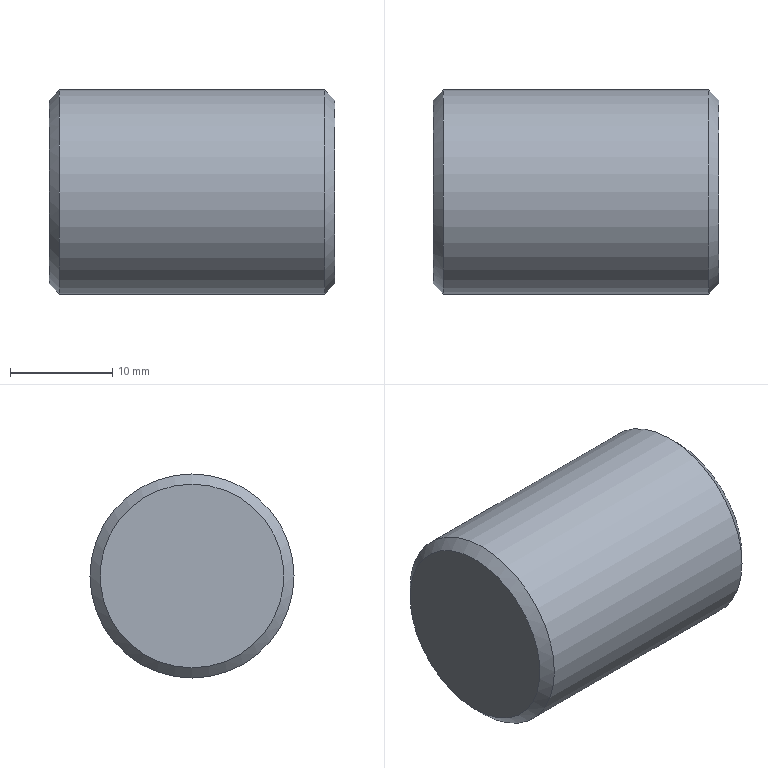Part | NX | features DATUM_CSYS 2, CHAMFER 1, EXTRUDE 1, SKETCH 1 | 1 solid | 5 faces | box 28 x 20 x 20 mm | volume 8736 mm3 | plane 2 | cone 2 | cylinder 1 | commonest cylinder face diameters 20 x1
STEP:
#1=CARTESIAN_POINT('',(-13.,0.,-10.));
#2=VERTEX_POINT('',#1);
#3=CARTESIAN_POINT('',(-13.,0.,0.));
#4=DIRECTION('',(1.,0.,0.));
#5=DIRECTION('',(0.,0.,-1.));
#6=AXIS2_PLACEMENT_3D('',#3,#4,#5);
#7=CIRCLE('',#6,10.);
#8=EDGE_CURVE('',#2,#2,#7,.T.);
#9=ORIENTED_EDGE('',*,*,#8,.T.);
#10=EDGE_LOOP('',(#9));
#11=FACE_BOUND('',#10,.T.);
#12=CARTESIAN_POINT('',(13.,0.,-10.));
#13=VERTEX_POINT('',#12);
#14=CARTESIAN_POINT('',(13.,0.,0.));
#15=DIRECTION('',(1.,0.,0.));
#16=DIRECTION('',(0.,0.,-1.));
#17=AXIS2_PLACEMENT_3D('',#14,#15,#16);
#18=CIRCLE('',#17,10.);
#19=EDGE_CURVE('',#13,#13,#18,.F.);
#20=ORIENTED_EDGE('',*,*,#19,.T.);
#21=EDGE_LOOP('',(#20));
#22=FACE_BOUND('',#21,.T.);
#23=CARTESIAN_POINT('',(14.,0.,0.));
#24=DIRECTION('',(-1.,0.,0.));
#25=DIRECTION('',(0.,0.,1.));
#26=AXIS2_PLACEMENT_3D('',#23,#24,#25);
#27=CYLINDRICAL_SURFACE('',#26,10.);
#28=ADVANCED_FACE('',(#11,#22),#27,.T.);
#29=CARTESIAN_POINT('',(14.,0.,-9.));
#30=VERTEX_POINT('',#29);
#31=CARTESIAN_POINT('',(14.,0.,0.));
#32=DIRECTION('',(1.,0.,0.));
#33=DIRECTION('',(0.,0.,-1.));
#34=AXIS2_PLACEMENT_3D('',#31,#32,#33);
#35=CIRCLE('',#34,9.);
#36=EDGE_CURVE('',#30,#30,#35,.T.);
#37=ORIENTED_EDGE('',*,*,#36,.T.);
#38=EDGE_LOOP('',(#37));
#39=FACE_BOUND('',#38,.T.);
#40=CARTESIAN_POINT('',(14.,0.,0.));
#41=DIRECTION('',(1.,0.,0.));
#42=DIRECTION('',(0.,0.,-1.));
#43=AXIS2_PLACEMENT_3D('',#40,#41,#42);
#44=PLANE('',#43);
#45=ADVANCED_FACE('',(#39),#44,.T.);
#46=CARTESIAN_POINT('',(-14.,0.,-9.));
#47=VERTEX_POINT('',#46);
#48=CARTESIAN_POINT('',(-14.,0.,0.));
#49=DIRECTION('',(1.,0.,0.));
#50=DIRECTION('',(0.,0.,-1.));
#51=AXIS2_PLACEMENT_3D('',#48,#49,#50);
#52=CIRCLE('',#51,9.);
#53=EDGE_CURVE('',#47,#47,#52,.F.);
#54=ORIENTED_EDGE('',*,*,#53,.T.);
#55=EDGE_LOOP('',(#54));
#56=FACE_BOUND('',#55,.T.);
#57=CARTESIAN_POINT('',(-14.,0.,0.));
#58=DIRECTION('',(1.,0.,0.));
#59=DIRECTION('',(0.,0.,-1.));
#60=AXIS2_PLACEMENT_3D('',#57,#58,#59);
#61=PLANE('',#60);
#62=ADVANCED_FACE('',(#56),#61,.F.);
#63=ORIENTED_EDGE('',*,*,#53,.F.);
#64=EDGE_LOOP('',(#63));
#65=FACE_BOUND('',#64,.T.);
#66=ORIENTED_EDGE('',*,*,#8,.F.);
#67=EDGE_LOOP('',(#66));
#68=FACE_BOUND('',#67,.T.);
#69=CARTESIAN_POINT('',(-13.,0.,0.));
#70=DIRECTION('',(1.,0.,0.));
#71=DIRECTION('',(0.,0.,-1.));
#72=AXIS2_PLACEMENT_3D('',#69,#70,#71);
#73=CONICAL_SURFACE('',#72,10.,0.7854);
#74=ADVANCED_FACE('',(#65,#68),#73,.T.);
#75=ORIENTED_EDGE('',*,*,#19,.F.);
#76=EDGE_LOOP('',(#75));
#77=FACE_BOUND('',#76,.T.);
#78=ORIENTED_EDGE('',*,*,#36,.F.);
#79=EDGE_LOOP('',(#78));
#80=FACE_BOUND('',#79,.T.);
#81=CARTESIAN_POINT('',(14.,0.,0.));
#82=DIRECTION('',(-1.,0.,0.));
#83=DIRECTION('',(0.,0.,1.));
#84=AXIS2_PLACEMENT_3D('',#81,#82,#83);
#85=CONICAL_SURFACE('',#84,9.,0.7854);
#86=ADVANCED_FACE('',(#77,#80),#85,.T.);
#87=CLOSED_SHELL('',(#28,#45,#62,#74,#86));
#88=MANIFOLD_SOLID_BREP('',#87);
#89=(LENGTH_UNIT()NAMED_UNIT(*)SI_UNIT(.MILLI.,.METRE.));
#90=UNCERTAINTY_MEASURE_WITH_UNIT(LENGTH_MEASURE(0.00001),#89,'','');
#91=(NAMED_UNIT(*)PLANE_ANGLE_UNIT()SI_UNIT($,.RADIAN.));
#92=(NAMED_UNIT(*)SI_UNIT($,.STERADIAN.)SOLID_ANGLE_UNIT());
#93=(GEOMETRIC_REPRESENTATION_CONTEXT(3)GLOBAL_UNCERTAINTY_ASSIGNED_CONTEXT((#90))GLOBAL_UNIT_ASSIGNED_CONTEXT((#89,#91,#92))REPRESENTATION_CONTEXT('',''));
#94=ADVANCED_BREP_SHAPE_REPRESENTATION('',(#88),#93);